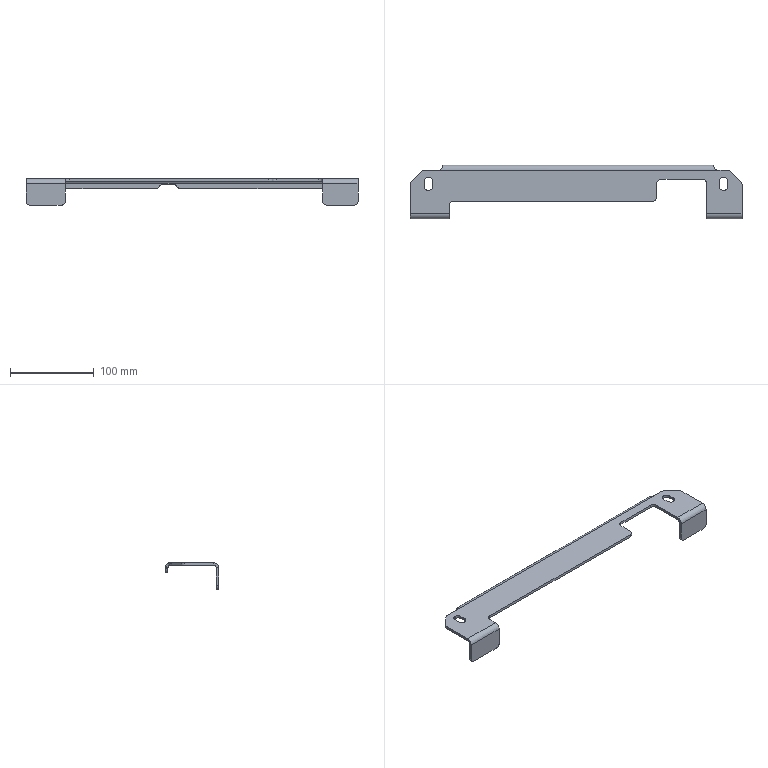Part | SolidWorks | features ICE 2, Fillet 1, FlatPattern 1, Fold 1, SMBaseFlange 1, SheetMetal 1, UnFold 1 | 1 solid | 74 faces | box 397 x 64 x 32 mm | volume 66915 mm3 | plane 42 | cylinder 30 | spline 2 | commonest cylinder face diameters 10 x24 6 x3 12.4 x3